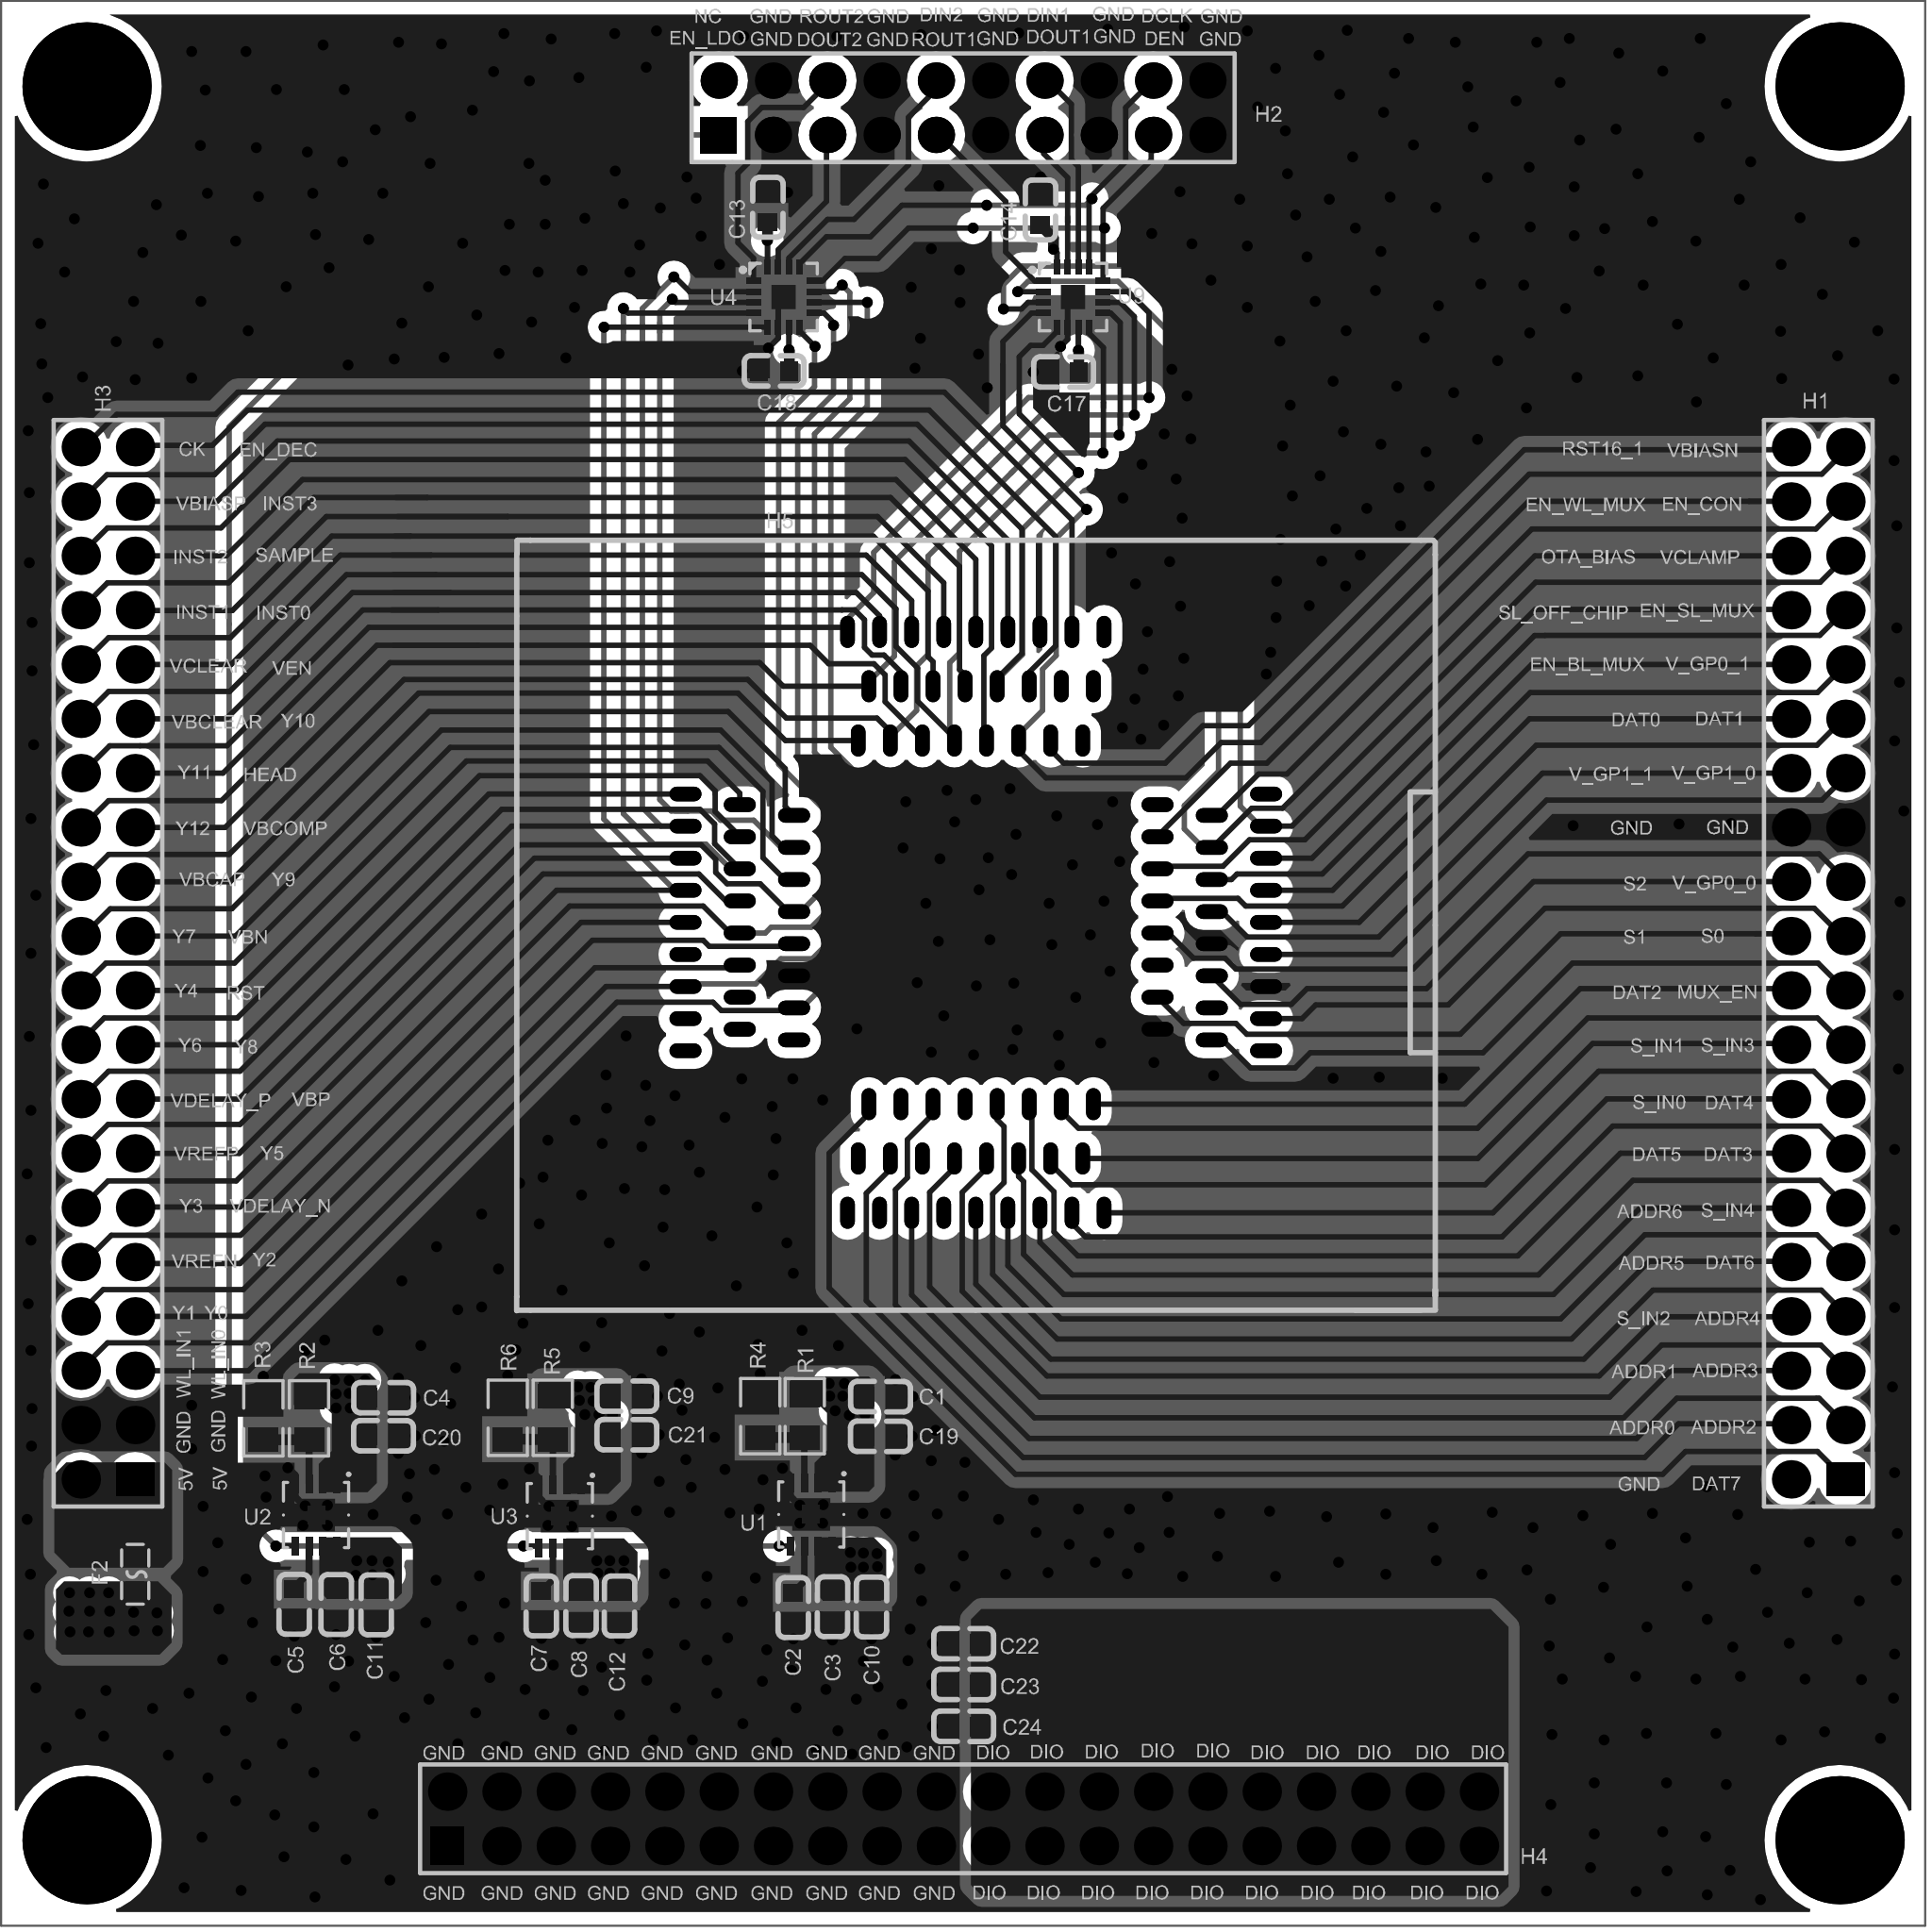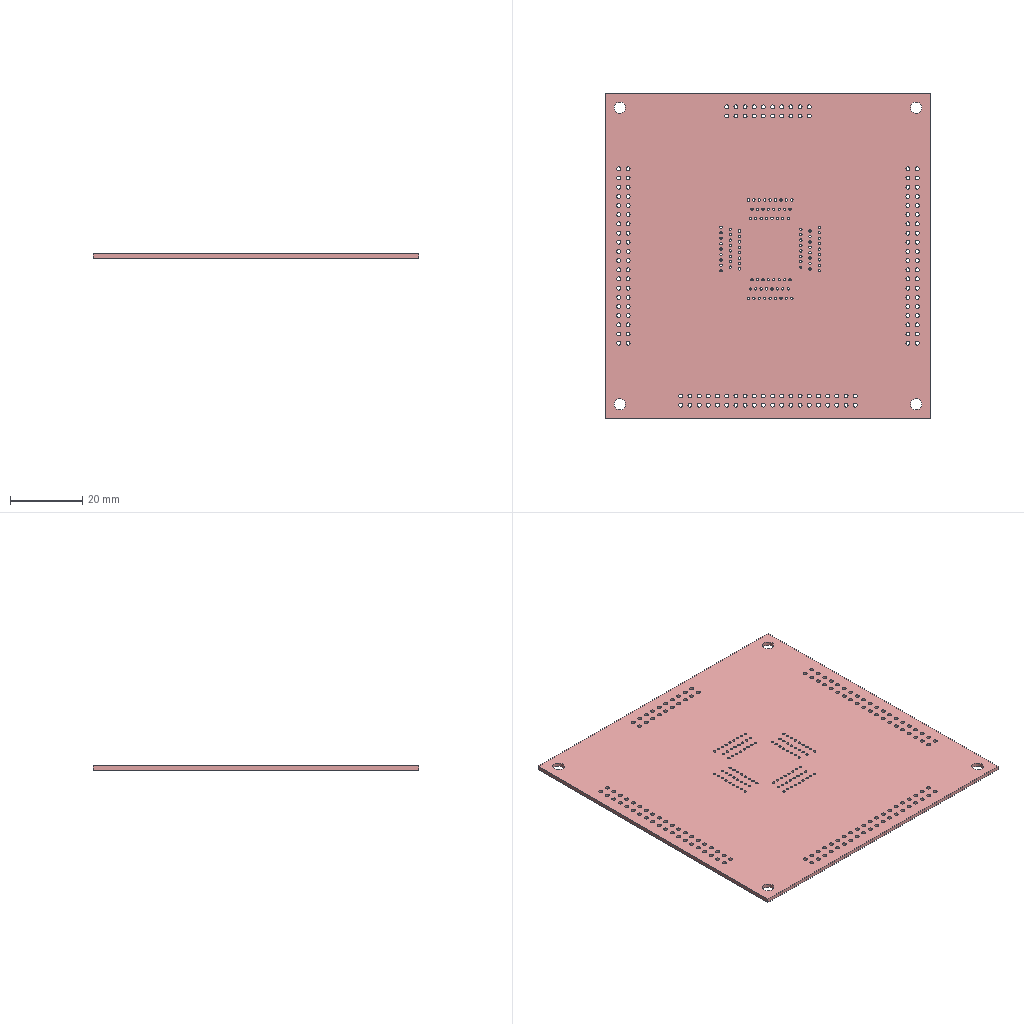Circuit board layout | Altium Designer | box 90 x 90 x 1.1 mm
Layer stack:
# Altium Designer layer stack of  (unit mm; dielectric type: 0 none, 1 core, 2 prepreg, 3 surface material)
index,name,kind,layer,copper_thickness_mm,dielectric_type,dielectric_thickness_mm,dielectric_material,dielectric_constant
0,Top Paste,other,,,,,,
1,Top Overlay,other,,,,,,
2,Top Solder,dielectric,,,3,0.0102,Solder Resist,3.5
3,Top Layer,copper,Top Layer,0.0356,,,,
4,Dielectric1,dielectric,,,1,0.32,FR-4,4.8
5,GND,copper,GND,0.0356,,,,
6,Dielectric5,dielectric,,,2,0.32,FR-4,4.8
7,POWER,copper,POWER,0.0356,,,,
8,Dielectric6,dielectric,,,1,0.32,FR-4,4.8
9,Bottom Layer,copper,Bottom Layer,0.0356,,,,
10,Bottom Solder,dielectric,,,3,0.0102,Solder Resist,3.5
11,Bottom Overlay,other,,,,,,
12,Bottom Paste,other,,,,,,
# drill layer pairs: low layer,high layer
drill_pair,Top Layer,Bottom Layer
Part placement:
Designator,Comment,Layer,Footprint,Center-X(mm),Center-Y(mm),Rotation
C1,4.7uF/16V,TopLayer,C0603,41.129,24.741,180
C2,10nF/16V,TopLayer,C0603,37.059,14.884,90
C3,1uF/16V,TopLayer,C0603,38.887,14.91,270
C4,4.7uF/16V,TopLayer,C0603,17.888,24.69,180
C5,10nF/16V,TopLayer,C0603,13.716,15.037,90
C6,1uF/16V,TopLayer,C0603,15.672,15.011,270
C7,10nF/16V,TopLayer,C0603,25.273,14.961,90
C8,1uF/16V,TopLayer,C0603,27.127,14.961,270
C9,4.7uF/16V,TopLayer,C0603,29.261,24.765,180
F2,BSMD0603-050-6V,TopLayer,F0603,6.274,16.434,90
H1,12251220ANG0S115001,TopLayer,HDR-TH_40P-P2.54-V-M-R2-C20-S2.54,85,45,90
H4,12251220ANG0S115001,TopLayer,HDR-TH_40P-P2.54-V-M-R2-C20-S2.54,45,5,0
H2,PZ254V-12-20P,TopLayer,HDR-TH_20P-P2.54-V-M-R2-C10-S2.54,45,85,360
H3,12251220ANG0S115001,TopLayer,HDR-TH_40P-P2.54-V-M-R2-C20-S2.54,5,45,90
H5,220-1S-2*50PStraight row of mothersH=4.3 Gold-plated,TopLayer,IC51-1004-809-23,45.593,46.914,90
R1,1.25k,TopLayer,R0805,37.592,23.825,270
R3,10k,TopLayer,R0805,12.268,23.724,270
R4,10k,TopLayer,R0805,35.509,23.825,270
R6,10k,TopLayer,R0805,23.698,23.749,270
R2,12.4k,TopLayer,R0805,14.402,23.724,270
R5,12.4k,TopLayer,R0805,25.806,23.749,270
U1,TPS7A8001DRBR,TopLayer,VSON-8_L3.0-W3.0-P0.65-TL-EP,37.897,19.228,270
U2,TPS7A8001DRBR,TopLayer,VSON-8_L3.0-W3.0-P0.65-TL-EP,14.732,19.202,270
U3,TPS7A8001DRBR,TopLayer,VSON-8_L3.0-W3.0-P0.65-TL-EP,26.137,19.152,270
U4,DAC60508ZRTER,TopLayer,WQFN-16_L3.0-W3.0-P0.50-BL-EP0.8,36.601,76.149,270
U9,DAC60508ZRTER,TopLayer,WQFN-16_L3.0-W3.0-P0.50-BL-EP0.8,50.14,76.149,270
C10,4.7uF/16V,TopLayer,C0603,40.716,14.91,90
C11,4.7uF/16V,TopLayer,C0603,17.551,15.011,90
C12,4.7uF/16V,TopLayer,C0603,28.931,14.961,90
C13,0.1uF/16V,TopLayer,C0603,35.865,80.34,270
C14,0.1uF/16V,TopLayer,C0603,48.616,80.213,270
C17,0.1uF/16V,TopLayer,C0603,49.708,72.644,360
C18,0.1uF/16V,TopLayer,C0603,36.17,72.695,360
C19,4.7uF/16V,TopLayer,C0603,41.123,22.885,180
C20,4.7uF/16V,TopLayer,C0603,17.882,22.911,180
C21,4.7uF/16V,TopLayer,C0603,29.261,22.962,180
C22,4.7uF/16V,TopLayer,C0603,45.034,13.183,360
C23,4.7uF/16V,TopLayer,C0603,45.034,11.278,360
C24,4.7uF/16V,TopLayer,C0603,45.034,9.322,360
Pad and via stacks:
# Altium Designer via and pad stacks of  (unit mm). Each distinct definition once, with the count of objects using it.
# via: kind,start_layer,end_layer,hole_mm,diameter_mm,mode(0 simple;1 top-mid-bottom;2 full stack),diameter_per_layer,count,example_net
# pad: kind,layer,hole_mm,hole_type(0 round;1 square;2 slot),plating,top_size,top_shape(1 round;2 rect;3 octagon;9 rounded rect),mid_size,bottom_size,mode,footprint,size_per_layer,count,example
pad,Top Layer,0,0,plated,0.8x0.9,2,0.8x0.9,0.8x0.9,0,C0603,,44,C1.2
pad,Top Layer,0,0,plated,1.133x1.377,2,1.133x1.377,1.133x1.377,0,R0805,,12,R1.2
pad,Top Layer,0,0,plated,0.28x0.665,2,0.28x0.665,0.28x0.665,0,WQFN-16_L3.0-W3.0-P0.50-BL-EP0.8,,16,U4.1
pad,Top Layer,0,0,plated,0.665x0.28,2,0.665x0.28,0.665x0.28,0,WQFN-16_L3.0-W3.0-P0.50-BL-EP0.8,,16,U4.5
pad,Top Layer,0,0,plated,0.8x0.8,2,0.8x0.8,0.8x0.8,0,WQFN-16_L3.0-W3.0-P0.50-BL-EP0.8,,2,U4.17
pad,Top Layer,0,0,plated,0.8065x0.864,2,0.8065x0.864,0.8065x0.864,0,F0603,,2,F2.2
pad,Top Layer,0,0,plated,0.34x0.8499,2,0.34x0.8499,0.34x0.8499,0,VSON-8_L3.0-W3.0-P0.65-TL-EP,,24,U3.8
pad,Top Layer,0,0,plated,0.8382x0.8382,2,0.8382x0.8382,0.8382x0.8382,0,VSON-8_L3.0-W3.0-P0.65-TL-EP,,3,U3.9
pad,Multi-Layer,1.1,0,plated,1.7x1.7,1,1.7x1.7,1.7x1.7,0,HDR-TH_20P-P2.54-V-M-R2-C10-S2.54,,19,H2.20
pad,Multi-Layer,1.1,0,plated,1.7x1.7,2,1.7x1.7,1.7x1.7,0,HDR-TH_20P-P2.54-V-M-R2-C10-S2.54,,1,H2.1
pad,Multi-Layer,0.65,0,plated,0.6858x1.5,1,0.6858x1.5,0.6858x1.5,0,IC51-1004-809-23,,49,H5.44
pad,Multi-Layer,0.65,0,plated,1.5x0.6858,1,1.5x0.6858,1.5x0.6858,0,IC51-1004-809-23,,49,H5.51
pad,Multi-Layer,0.61,0,plated,1.5x0.6858,1,1.5x0.6858,1.5x0.6858,0,IC51-1004-809-23,,1,H5.2
pad,Multi-Layer,0.61,0,plated,0.6858x1.5,1,0.6858x1.5,0.6858x1.5,0,IC51-1004-809-23,,1,H5.28
pad,Multi-Layer,1.1,0,plated,1.8x1.8,1,1.524x1.524,1.524x1.524,1,HDR-TH_40P-P2.54-V-M-R2-C20-S2.54,,117,H1.40
pad,Multi-Layer,1.1,0,plated,1.575x1.8,2,1.524x1.524,1.524x1.524,1,HDR-TH_40P-P2.54-V-M-R2-C20-S2.54,,3,H1.1
pad,Multi-Layer,3.2,0,plated,6x6,1,6x6,6x6,0,,,4,0
via,Top Layer,Bottom Layer,0.3048,0.508,0,,705,GND
Copper pours:
name,layer,net,type(0 solid;1 hatched;2 none)
Bottom Layer-No Net,Top Layer,GND,0
Bottom Layer-No Net,Top Layer,DVDDIO,0
Bottom Layer-No Net,Top Layer,DVDD,0
Bottom Layer-No Net,Top Layer,5.0V,0
Bottom Layer-No Net,Top Layer,5V,0
Bottom Layer-No Net,Top Layer,5V,0
Bottom Layer-No Net,Top Layer,DVDDIO,0
Bottom Layer-No Net,Top Layer,5V,0
Bottom Layer-No Net,Top Layer,AVDD,0
Bottom Layer-No Net,Top Layer,5V,0
Bottom Layer-No Net,Bottom Layer,GND,0
Design rules, without the lines most boards share:
# Altium Designer design rules of  (exported by Altium Designer, unit mm)
# columns: name | kind | enabled | priority | scope1 | scope2 | descriptor | typed fields (field=value)
Clearance_1 | 0 | enabled | 1 | INPOLYGON | All | Clearance Constraint (Gap=6mil) (INPOLYGON),(All) | gap=0.1524
Clearance | 0 | enabled | 2 | All | All | Clearance Constraint (Gap=6mil) (All),(All) | gap=0.1524
PlaneConnect | 6 | enabled | 1 | All | All | Power Plane Connect Rule(Direct Connect )(Expansion=20mil) (Conductor Width=10mil) (Air Gap=10mil) (Entries=4) (All) | relief_conductor_width=0.254 relief_entries=4 relief_expansion=0.508
PlaneClearance | 12 | enabled | 1 | All | All | Power Plane Clearance (Clearance =6mil) (All) | clearance=0.1524
PolygonConnect | 20 | enabled | 1 | All | All | Polygon Connect Rule(Direct Connect )(Conductor Width=10mil) (Relief Angle=90 Angle) (Entries=4) (Air Gap Width=10mil) (All),(All) | connect_style(0=relief,1=direct,2=none)=1 relief_conductor_width=0.254 relief_entries=4
Width | 2 | enabled | 1 | All | All | Width Constraint (Min=10mil) (Max=40mil) (Preferred=10mil) (All) |
RoutingVias | 11 | enabled | 1 | All | All | Routing Via (MinHoleWidth=12mil) (MaxHoleWidth=12mil) (PreferredHoleWidth=12mil) (MinWidth=20mil) (MaxWidth=20mil) (PreferedWidth=20mil) (All) | via_min_hole=0.3048 via_max_hole=0.3048 via_preferred_diameter=0.508 via_preferred_hole=0.3048
SolderMaskExpansion | 13 | enabled | 1 | All | All | Solder Mask Expansion (Expansion =4mil) (All) | expansion=0.1016
HoleSize | 42 | enabled | 1 | All | All | Hole Size Constraint (Min=1mil) (Max=500mil) (All) |
DiffPairsRouting | 51 | enabled | 1 | All | All | Differential Pairs Uncoupled Length using the Gap Constraints (Min=10mil) (Max=10mil) (Prefered=10mil)  and Width Constraints (Min=15mil) (Max=15mil) (Prefered=15mil) (All) |
HoleToHoleClearance | 52 | enabled | 1 | All | All | Hole To Hole Clearance (Gap=0mil) (All),(All) | gap=0
MinimumSolderMaskSliver | 53 | enabled | 1 | All | All | Minimum Solder Mask Sliver (Gap=0mil) (All),(All) |
SilkscreenOverComponentPads | 54 | enabled | 1 | IsPad | All | Silk To Solder Mask (Clearance=0mil) (IsPad),(All) |
SilkToSilkClearance | 55 | enabled | 1 | All | All | Silk to Silk (Clearance=0mil) (All),(All) |